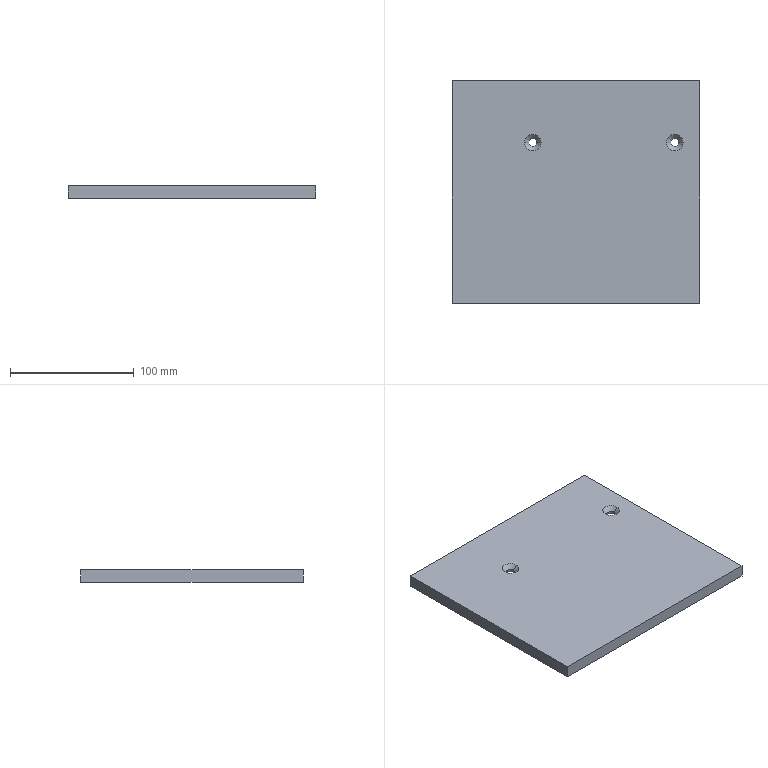Part | STEP file | 001-004-Feeding mechanism shaft slideway base plate | 1 solid | 20 faces | box 200 x 180 x 10 mm | volume 352263 mm3 | cylinder 8 | plane 8 | cone 4 | commonest cylinder face diameters 6.6 x4 30 x4
STEP:
#1=CARTESIAN_POINT('',(0.,0.,0.));
#2=DIRECTION('',(0.,0.,1.));
#3=DIRECTION('',(1.,0.,0.));
#4=AXIS2_PLACEMENT_3D('',#1,#2,#3);
#5=CARTESIAN_POINT('',(-31.7,40.,6.58));
#6=VERTEX_POINT('',#5);
#7=CARTESIAN_POINT('',(-28.28,40.,10.));
#8=VERTEX_POINT('',#7);
#9=CARTESIAN_POINT('',(-28.28,40.,10.));
#10=DIRECTION('',(0.7071,0.,0.7071));
#11=VECTOR('',#10,1.);
#12=LINE('',#9,#11);
#13=CARTESIAN_POINT('',(-35.,40.,10.));
#14=DIRECTION('',(0.,0.,1.));
#15=DIRECTION('',(1.,0.,0.));
#16=AXIS2_PLACEMENT_3D('',#13,#14,#15);
#17=CONICAL_SURFACE('',#16,6.72,0.7854);
#18=CARTESIAN_POINT('',(6.283,0.));
#19=DIRECTION('',(0.,1.));
#20=VECTOR('',#19,1.);
#21=LINE('',#18,#20);
#22=(GEOMETRIC_REPRESENTATION_CONTEXT(2)PARAMETRIC_REPRESENTATION_CONTEXT()REPRESENTATION_CONTEXT('',''));
#23=DEFINITIONAL_REPRESENTATION('',(#21),#22);
#24=PCURVE('',#17,#23);
#25=CARTESIAN_POINT('',(-35.,40.,10.));
#26=DIRECTION('',(0.,0.,1.));
#27=DIRECTION('',(1.,0.,0.));
#28=AXIS2_PLACEMENT_3D('',#25,#26,#27);
#29=CONICAL_SURFACE('',#28,6.72,0.7854);
#30=CARTESIAN_POINT('',(0.,0.));
#31=DIRECTION('',(0.,1.));
#32=VECTOR('',#31,1.);
#33=LINE('',#30,#32);
#34=(GEOMETRIC_REPRESENTATION_CONTEXT(2)PARAMETRIC_REPRESENTATION_CONTEXT()REPRESENTATION_CONTEXT('',''));
#35=DEFINITIONAL_REPRESENTATION('',(#33),#34);
#36=PCURVE('',#29,#35);
#37=SURFACE_CURVE('',#12,(#24,#36),.PCURVE_S1.);
#38=EDGE_CURVE('',#6,#8,#37,.T.);
#39=ORIENTED_EDGE('',*,*,#38,.T.);
#40=CARTESIAN_POINT('',(-41.72,40.,10.));
#41=VERTEX_POINT('',#40);
#42=CARTESIAN_POINT('',(-35.,40.,10.));
#43=DIRECTION('',(0.,0.,1.));
#44=DIRECTION('',(1.,0.,0.));
#45=AXIS2_PLACEMENT_3D('',#42,#43,#44);
#46=CIRCLE('',#45,6.72);
#47=CARTESIAN_POINT('',(0.,0.));
#48=DIRECTION('',(1.,0.));
#49=VECTOR('',#48,1.);
#50=LINE('',#47,#49);
#51=(GEOMETRIC_REPRESENTATION_CONTEXT(2)PARAMETRIC_REPRESENTATION_CONTEXT()REPRESENTATION_CONTEXT('',''));
#52=DEFINITIONAL_REPRESENTATION('',(#50),#51);
#53=PCURVE('',#17,#52);
#54=CARTESIAN_POINT('',(0.,0.,10.));
#55=DIRECTION('',(0.,0.,1.));
#56=DIRECTION('',(1.,0.,0.));
#57=AXIS2_PLACEMENT_3D('',#54,#55,#56);
#58=PLANE('',#57);
#59=CARTESIAN_POINT('',(-35.,40.));
#60=DIRECTION('',(1.,0.));
#61=AXIS2_PLACEMENT_2D('',#59,#60);
#62=CIRCLE('',#61,6.72);
#63=(GEOMETRIC_REPRESENTATION_CONTEXT(2)PARAMETRIC_REPRESENTATION_CONTEXT()REPRESENTATION_CONTEXT('',''));
#64=DEFINITIONAL_REPRESENTATION('',(#62),#63);
#65=PCURVE('',#58,#64);
#66=SURFACE_CURVE('',#46,(#53,#65),.PCURVE_S1.);
#67=EDGE_CURVE('',#41,#8,#66,.T.);
#68=ORIENTED_EDGE('',*,*,#67,.F.);
#69=CARTESIAN_POINT('',(-38.3,40.,6.58));
#70=VERTEX_POINT('',#69);
#71=CARTESIAN_POINT('',(-41.72,40.,10.));
#72=DIRECTION('',(-0.7071,0.,0.7071));
#73=VECTOR('',#72,1.);
#74=LINE('',#71,#73);
#75=CARTESIAN_POINT('',(3.142,0.));
#76=DIRECTION('',(0.,1.));
#77=VECTOR('',#76,1.);
#78=LINE('',#75,#77);
#79=(GEOMETRIC_REPRESENTATION_CONTEXT(2)PARAMETRIC_REPRESENTATION_CONTEXT()REPRESENTATION_CONTEXT('',''));
#80=DEFINITIONAL_REPRESENTATION('',(#78),#79);
#81=PCURVE('',#17,#80);
#82=CARTESIAN_POINT('',(3.142,0.));
#83=DIRECTION('',(0.,1.));
#84=VECTOR('',#83,1.);
#85=LINE('',#82,#84);
#86=(GEOMETRIC_REPRESENTATION_CONTEXT(2)PARAMETRIC_REPRESENTATION_CONTEXT()REPRESENTATION_CONTEXT('',''));
#87=DEFINITIONAL_REPRESENTATION('',(#85),#86);
#88=PCURVE('',#29,#87);
#89=SURFACE_CURVE('',#74,(#81,#88),.PCURVE_S1.);
#90=EDGE_CURVE('',#70,#41,#89,.T.);
#91=ORIENTED_EDGE('',*,*,#90,.F.);
#92=CARTESIAN_POINT('',(-35.,40.,6.58));
#93=DIRECTION('',(0.,0.,1.));
#94=DIRECTION('',(1.,0.,0.));
#95=AXIS2_PLACEMENT_3D('',#92,#93,#94);
#96=CIRCLE('',#95,3.3);
#97=CARTESIAN_POINT('',(0.,-3.42));
#98=DIRECTION('',(1.,0.));
#99=VECTOR('',#98,1.);
#100=LINE('',#97,#99);
#101=(GEOMETRIC_REPRESENTATION_CONTEXT(2)PARAMETRIC_REPRESENTATION_CONTEXT()REPRESENTATION_CONTEXT('',''));
#102=DEFINITIONAL_REPRESENTATION('',(#100),#101);
#103=PCURVE('',#17,#102);
#104=CARTESIAN_POINT('',(-35.,40.,10.));
#105=DIRECTION('',(0.,0.,1.));
#106=DIRECTION('',(1.,0.,0.));
#107=AXIS2_PLACEMENT_3D('',#104,#105,#106);
#108=CYLINDRICAL_SURFACE('',#107,3.3);
#109=CARTESIAN_POINT('',(0.,-3.42));
#110=DIRECTION('',(1.,0.));
#111=VECTOR('',#110,1.);
#112=LINE('',#109,#111);
#113=(GEOMETRIC_REPRESENTATION_CONTEXT(2)PARAMETRIC_REPRESENTATION_CONTEXT()REPRESENTATION_CONTEXT('',''));
#114=DEFINITIONAL_REPRESENTATION('',(#112),#113);
#115=PCURVE('',#108,#114);
#116=SURFACE_CURVE('',#96,(#103,#115),.PCURVE_S1.);
#117=EDGE_CURVE('',#70,#6,#116,.T.);
#118=ORIENTED_EDGE('',*,*,#117,.T.);
#119=EDGE_LOOP('',(#39,#68,#91,#118));
#120=FACE_BOUND('',#119,.F.);
#121=ADVANCED_FACE('',(#120),#17,.F.);
#122=CARTESIAN_POINT('',(-31.7,40.,5.));
#123=VERTEX_POINT('',#122);
#124=CARTESIAN_POINT('',(-31.7,40.,10.));
#125=DIRECTION('',(0.,0.,1.));
#126=VECTOR('',#125,1.);
#127=LINE('',#124,#126);
#128=CARTESIAN_POINT('',(6.283,0.));
#129=DIRECTION('',(0.,1.));
#130=VECTOR('',#129,1.);
#131=LINE('',#128,#130);
#132=(GEOMETRIC_REPRESENTATION_CONTEXT(2)PARAMETRIC_REPRESENTATION_CONTEXT()REPRESENTATION_CONTEXT('',''));
#133=DEFINITIONAL_REPRESENTATION('',(#131),#132);
#134=PCURVE('',#108,#133);
#135=CARTESIAN_POINT('',(-35.,40.,10.));
#136=DIRECTION('',(0.,0.,1.));
#137=DIRECTION('',(1.,0.,0.));
#138=AXIS2_PLACEMENT_3D('',#135,#136,#137);
#139=CYLINDRICAL_SURFACE('',#138,3.3);
#140=CARTESIAN_POINT('',(0.,0.));
#141=DIRECTION('',(0.,1.));
#142=VECTOR('',#141,1.);
#143=LINE('',#140,#142);
#144=(GEOMETRIC_REPRESENTATION_CONTEXT(2)PARAMETRIC_REPRESENTATION_CONTEXT()REPRESENTATION_CONTEXT('',''));
#145=DEFINITIONAL_REPRESENTATION('',(#143),#144);
#146=PCURVE('',#139,#145);
#147=SURFACE_CURVE('',#127,(#134,#146),.PCURVE_S1.);
#148=EDGE_CURVE('',#123,#6,#147,.T.);
#149=ORIENTED_EDGE('',*,*,#148,.T.);
#150=ORIENTED_EDGE('',*,*,#117,.F.);
#151=CARTESIAN_POINT('',(-38.3,40.,5.));
#152=VERTEX_POINT('',#151);
#153=CARTESIAN_POINT('',(-38.3,40.,10.));
#154=DIRECTION('',(0.,0.,1.));
#155=VECTOR('',#154,1.);
#156=LINE('',#153,#155);
#157=CARTESIAN_POINT('',(3.142,0.));
#158=DIRECTION('',(0.,1.));
#159=VECTOR('',#158,1.);
#160=LINE('',#157,#159);
#161=(GEOMETRIC_REPRESENTATION_CONTEXT(2)PARAMETRIC_REPRESENTATION_CONTEXT()REPRESENTATION_CONTEXT('',''));
#162=DEFINITIONAL_REPRESENTATION('',(#160),#161);
#163=PCURVE('',#108,#162);
#164=CARTESIAN_POINT('',(3.142,0.));
#165=DIRECTION('',(0.,1.));
#166=VECTOR('',#165,1.);
#167=LINE('',#164,#166);
#168=(GEOMETRIC_REPRESENTATION_CONTEXT(2)PARAMETRIC_REPRESENTATION_CONTEXT()REPRESENTATION_CONTEXT('',''));
#169=DEFINITIONAL_REPRESENTATION('',(#167),#168);
#170=PCURVE('',#139,#169);
#171=SURFACE_CURVE('',#156,(#163,#170),.PCURVE_S1.);
#172=EDGE_CURVE('',#152,#70,#171,.T.);
#173=ORIENTED_EDGE('',*,*,#172,.F.);
#174=CARTESIAN_POINT('',(-35.,40.,5.));
#175=DIRECTION('',(0.,0.,-1.));
#176=DIRECTION('',(-1.,0.,0.));
#177=AXIS2_PLACEMENT_3D('',#174,#175,#176);
#178=CIRCLE('',#177,3.3);
#179=CARTESIAN_POINT('',(9.425,-5.));
#180=DIRECTION('',(-1.,0.));
#181=VECTOR('',#180,1.);
#182=LINE('',#179,#181);
#183=(GEOMETRIC_REPRESENTATION_CONTEXT(2)PARAMETRIC_REPRESENTATION_CONTEXT()REPRESENTATION_CONTEXT('',''));
#184=DEFINITIONAL_REPRESENTATION('',(#182),#183);
#185=PCURVE('',#108,#184);
#186=CARTESIAN_POINT('',(-35.,40.,5.));
#187=DIRECTION('',(0.,0.,-1.));
#188=DIRECTION('',(-1.,0.,0.));
#189=AXIS2_PLACEMENT_3D('',#186,#187,#188);
#190=PLANE('',#189);
#191=CARTESIAN_POINT('',(0.,0.));
#192=DIRECTION('',(1.,0.));
#193=AXIS2_PLACEMENT_2D('',#191,#192);
#194=CIRCLE('',#193,3.3);
#195=(GEOMETRIC_REPRESENTATION_CONTEXT(2)PARAMETRIC_REPRESENTATION_CONTEXT()REPRESENTATION_CONTEXT('',''));
#196=DEFINITIONAL_REPRESENTATION('',(#194),#195);
#197=PCURVE('',#190,#196);
#198=SURFACE_CURVE('',#178,(#185,#197),.PCURVE_S1.);
#199=EDGE_CURVE('',#123,#152,#198,.T.);
#200=ORIENTED_EDGE('',*,*,#199,.F.);
#201=EDGE_LOOP('',(#149,#150,#173,#200));
#202=FACE_BOUND('',#201,.F.);
#203=ADVANCED_FACE('',(#202),#108,.F.);
#204=CARTESIAN_POINT('',(83.3,40.,6.58));
#205=VERTEX_POINT('',#204);
#206=CARTESIAN_POINT('',(86.72,40.,10.));
#207=VERTEX_POINT('',#206);
#208=CARTESIAN_POINT('',(86.72,40.,10.));
#209=DIRECTION('',(0.7071,0.,0.7071));
#210=VECTOR('',#209,1.);
#211=LINE('',#208,#210);
#212=CARTESIAN_POINT('',(80.,40.,10.));
#213=DIRECTION('',(0.,0.,1.));
#214=DIRECTION('',(1.,0.,0.));
#215=AXIS2_PLACEMENT_3D('',#212,#213,#214);
#216=CONICAL_SURFACE('',#215,6.72,0.7854);
#217=CARTESIAN_POINT('',(6.283,0.));
#218=DIRECTION('',(0.,1.));
#219=VECTOR('',#218,1.);
#220=LINE('',#217,#219);
#221=(GEOMETRIC_REPRESENTATION_CONTEXT(2)PARAMETRIC_REPRESENTATION_CONTEXT()REPRESENTATION_CONTEXT('',''));
#222=DEFINITIONAL_REPRESENTATION('',(#220),#221);
#223=PCURVE('',#216,#222);
#224=CARTESIAN_POINT('',(80.,40.,10.));
#225=DIRECTION('',(0.,0.,1.));
#226=DIRECTION('',(1.,0.,0.));
#227=AXIS2_PLACEMENT_3D('',#224,#225,#226);
#228=CONICAL_SURFACE('',#227,6.72,0.7854);
#229=CARTESIAN_POINT('',(0.,0.));
#230=DIRECTION('',(0.,1.));
#231=VECTOR('',#230,1.);
#232=LINE('',#229,#231);
#233=(GEOMETRIC_REPRESENTATION_CONTEXT(2)PARAMETRIC_REPRESENTATION_CONTEXT()REPRESENTATION_CONTEXT('',''));
#234=DEFINITIONAL_REPRESENTATION('',(#232),#233);
#235=PCURVE('',#228,#234);
#236=SURFACE_CURVE('',#211,(#223,#235),.PCURVE_S1.);
#237=EDGE_CURVE('',#205,#207,#236,.T.);
#238=ORIENTED_EDGE('',*,*,#237,.T.);
#239=CARTESIAN_POINT('',(73.28,40.,10.));
#240=VERTEX_POINT('',#239);
#241=CARTESIAN_POINT('',(80.,40.,10.));
#242=DIRECTION('',(0.,0.,1.));
#243=DIRECTION('',(1.,0.,0.));
#244=AXIS2_PLACEMENT_3D('',#241,#242,#243);
#245=CIRCLE('',#244,6.72);
#246=CARTESIAN_POINT('',(0.,0.));
#247=DIRECTION('',(1.,0.));
#248=VECTOR('',#247,1.);
#249=LINE('',#246,#248);
#250=(GEOMETRIC_REPRESENTATION_CONTEXT(2)PARAMETRIC_REPRESENTATION_CONTEXT()REPRESENTATION_CONTEXT('',''));
#251=DEFINITIONAL_REPRESENTATION('',(#249),#250);
#252=PCURVE('',#216,#251);
#253=CARTESIAN_POINT('',(80.,40.));
#254=DIRECTION('',(1.,0.));
#255=AXIS2_PLACEMENT_2D('',#253,#254);
#256=CIRCLE('',#255,6.72);
#257=(GEOMETRIC_REPRESENTATION_CONTEXT(2)PARAMETRIC_REPRESENTATION_CONTEXT()REPRESENTATION_CONTEXT('',''));
#258=DEFINITIONAL_REPRESENTATION('',(#256),#257);
#259=PCURVE('',#58,#258);
#260=SURFACE_CURVE('',#245,(#252,#259),.PCURVE_S1.);
#261=EDGE_CURVE('',#240,#207,#260,.T.);
#262=ORIENTED_EDGE('',*,*,#261,.F.);
#263=CARTESIAN_POINT('',(76.7,40.,6.58));
#264=VERTEX_POINT('',#263);
#265=CARTESIAN_POINT('',(73.28,40.,10.));
#266=DIRECTION('',(-0.7071,0.,0.7071));
#267=VECTOR('',#266,1.);
#268=LINE('',#265,#267);
#269=CARTESIAN_POINT('',(3.142,0.));
#270=DIRECTION('',(0.,1.));
#271=VECTOR('',#270,1.);
#272=LINE('',#269,#271);
#273=(GEOMETRIC_REPRESENTATION_CONTEXT(2)PARAMETRIC_REPRESENTATION_CONTEXT()REPRESENTATION_CONTEXT('',''));
#274=DEFINITIONAL_REPRESENTATION('',(#272),#273);
#275=PCURVE('',#216,#274);
#276=CARTESIAN_POINT('',(3.142,0.));
#277=DIRECTION('',(0.,1.));
#278=VECTOR('',#277,1.);
#279=LINE('',#276,#278);
#280=(GEOMETRIC_REPRESENTATION_CONTEXT(2)PARAMETRIC_REPRESENTATION_CONTEXT()REPRESENTATION_CONTEXT('',''));
#281=DEFINITIONAL_REPRESENTATION('',(#279),#280);
#282=PCURVE('',#228,#281);
#283=SURFACE_CURVE('',#268,(#275,#282),.PCURVE_S1.);
#284=EDGE_CURVE('',#264,#240,#283,.T.);
#285=ORIENTED_EDGE('',*,*,#284,.F.);
#286=CARTESIAN_POINT('',(80.,40.,6.58));
#287=DIRECTION('',(0.,0.,1.));
#288=DIRECTION('',(1.,0.,0.));
#289=AXIS2_PLACEMENT_3D('',#286,#287,#288);
#290=CIRCLE('',#289,3.3);
#291=CARTESIAN_POINT('',(0.,-3.42));
#292=DIRECTION('',(1.,0.));
#293=VECTOR('',#292,1.);
#294=LINE('',#291,#293);
#295=(GEOMETRIC_REPRESENTATION_CONTEXT(2)PARAMETRIC_REPRESENTATION_CONTEXT()REPRESENTATION_CONTEXT('',''));
#296=DEFINITIONAL_REPRESENTATION('',(#294),#295);
#297=PCURVE('',#216,#296);
#298=CARTESIAN_POINT('',(80.,40.,10.));
#299=DIRECTION('',(0.,0.,1.));
#300=DIRECTION('',(1.,0.,0.));
#301=AXIS2_PLACEMENT_3D('',#298,#299,#300);
#302=CYLINDRICAL_SURFACE('',#301,3.3);
#303=CARTESIAN_POINT('',(0.,-3.42));
#304=DIRECTION('',(1.,0.));
#305=VECTOR('',#304,1.);
#306=LINE('',#303,#305);
#307=(GEOMETRIC_REPRESENTATION_CONTEXT(2)PARAMETRIC_REPRESENTATION_CONTEXT()REPRESENTATION_CONTEXT('',''));
#308=DEFINITIONAL_REPRESENTATION('',(#306),#307);
#309=PCURVE('',#302,#308);
#310=SURFACE_CURVE('',#290,(#297,#309),.PCURVE_S1.);
#311=EDGE_CURVE('',#264,#205,#310,.T.);
#312=ORIENTED_EDGE('',*,*,#311,.T.);
#313=EDGE_LOOP('',(#238,#262,#285,#312));
#314=FACE_BOUND('',#313,.F.);
#315=ADVANCED_FACE('',(#314),#216,.F.);
#316=CARTESIAN_POINT('',(83.3,40.,5.));
#317=VERTEX_POINT('',#316);
#318=CARTESIAN_POINT('',(83.3,40.,10.));
#319=DIRECTION('',(0.,0.,1.));
#320=VECTOR('',#319,1.);
#321=LINE('',#318,#320);
#322=CARTESIAN_POINT('',(6.283,0.));
#323=DIRECTION('',(0.,1.));
#324=VECTOR('',#323,1.);
#325=LINE('',#322,#324);
#326=(GEOMETRIC_REPRESENTATION_CONTEXT(2)PARAMETRIC_REPRESENTATION_CONTEXT()REPRESENTATION_CONTEXT('',''));
#327=DEFINITIONAL_REPRESENTATION('',(#325),#326);
#328=PCURVE('',#302,#327);
#329=CARTESIAN_POINT('',(80.,40.,10.));
#330=DIRECTION('',(0.,0.,1.));
#331=DIRECTION('',(1.,0.,0.));
#332=AXIS2_PLACEMENT_3D('',#329,#330,#331);
#333=CYLINDRICAL_SURFACE('',#332,3.3);
#334=CARTESIAN_POINT('',(0.,0.));
#335=DIRECTION('',(0.,1.));
#336=VECTOR('',#335,1.);
#337=LINE('',#334,#336);
#338=(GEOMETRIC_REPRESENTATION_CONTEXT(2)PARAMETRIC_REPRESENTATION_CONTEXT()REPRESENTATION_CONTEXT('',''));
#339=DEFINITIONAL_REPRESENTATION('',(#337),#338);
#340=PCURVE('',#333,#339);
#341=SURFACE_CURVE('',#321,(#328,#340),.PCURVE_S1.);
#342=EDGE_CURVE('',#317,#205,#341,.T.);
#343=ORIENTED_EDGE('',*,*,#342,.T.);
#344=ORIENTED_EDGE('',*,*,#311,.F.);
#345=CARTESIAN_POINT('',(76.7,40.,5.));
#346=VERTEX_POINT('',#345);
#347=CARTESIAN_POINT('',(76.7,40.,10.));
#348=DIRECTION('',(0.,0.,1.));
#349=VECTOR('',#348,1.);
#350=LINE('',#347,#349);
#351=CARTESIAN_POINT('',(3.142,0.));
#352=DIRECTION('',(0.,1.));
#353=VECTOR('',#352,1.);
#354=LINE('',#351,#353);
#355=(GEOMETRIC_REPRESENTATION_CONTEXT(2)PARAMETRIC_REPRESENTATION_CONTEXT()REPRESENTATION_CONTEXT('',''));
#356=DEFINITIONAL_REPRESENTATION('',(#354),#355);
#357=PCURVE('',#302,#356);
#358=CARTESIAN_POINT('',(3.142,0.));
#359=DIRECTION('',(0.,1.));
#360=VECTOR('',#359,1.);
#361=LINE('',#358,#360);
#362=(GEOMETRIC_REPRESENTATION_CONTEXT(2)PARAMETRIC_REPRESENTATION_CONTEXT()REPRESENTATION_CONTEXT('',''));
#363=DEFINITIONAL_REPRESENTATION('',(#361),#362);
#364=PCURVE('',#333,#363);
#365=SURFACE_CURVE('',#350,(#357,#364),.PCURVE_S1.);
#366=EDGE_CURVE('',#346,#264,#365,.T.);
#367=ORIENTED_EDGE('',*,*,#366,.F.);
#368=CARTESIAN_POINT('',(80.,40.,5.));
#369=DIRECTION('',(0.,0.,-1.));
#370=DIRECTION('',(-1.,0.,0.));
#371=AXIS2_PLACEMENT_3D('',#368,#369,#370);
#372=CIRCLE('',#371,3.3);
#373=CARTESIAN_POINT('',(9.425,-5.));
#374=DIRECTION('',(-1.,0.));
#375=VECTOR('',#374,1.);
#376=LINE('',#373,#375);
#377=(GEOMETRIC_REPRESENTATION_CONTEXT(2)PARAMETRIC_REPRESENTATION_CONTEXT()REPRESENTATION_CONTEXT('',''));
#378=DEFINITIONAL_REPRESENTATION('',(#376),#377);
#379=PCURVE('',#302,#378);
#380=CARTESIAN_POINT('',(80.,40.,5.));
#381=DIRECTION('',(0.,0.,-1.));
#382=DIRECTION('',(-1.,0.,0.));
#383=AXIS2_PLACEMENT_3D('',#380,#381,#382);
#384=PLANE('',#383);
#385=CARTESIAN_POINT('',(0.,0.));
#386=DIRECTION('',(1.,0.));
#387=AXIS2_PLACEMENT_2D('',#385,#386);
#388=CIRCLE('',#387,3.3);
#389=(GEOMETRIC_REPRESENTATION_CONTEXT(2)PARAMETRIC_REPRESENTATION_CONTEXT()REPRESENTATION_CONTEXT('',''));
#390=DEFINITIONAL_REPRESENTATION('',(#388),#389);
#391=PCURVE('',#384,#390);
#392=SURFACE_CURVE('',#372,(#379,#391),.PCURVE_S1.);
#393=EDGE_CURVE('',#317,#346,#392,.T.);
#394=ORIENTED_EDGE('',*,*,#393,.F.);
#395=EDGE_LOOP('',(#343,#344,#367,#394));
#396=FACE_BOUND('',#395,.F.);
#397=ADVANCED_FACE('',(#396),#302,.F.);
#398=CARTESIAN_POINT('',(-50.,40.,5.));
#399=VERTEX_POINT('',#398);
#400=CARTESIAN_POINT('',(-50.,40.,0.));
#401=VERTEX_POINT('',#400);
#402=CARTESIAN_POINT('',(-50.,40.,5.));
#403=DIRECTION('',(0.,0.,-1.));
#404=VECTOR('',#403,1.);
#405=LINE('',#402,#404);
#406=CARTESIAN_POINT('',(-35.,40.,5.));
#407=DIRECTION('',(0.,0.,-1.));
#408=DIRECTION('',(-1.,0.,0.));
#409=AXIS2_PLACEMENT_3D('',#406,#407,#408);
#410=CYLINDRICAL_SURFACE('',#409,15.);
#411=CARTESIAN_POINT('',(6.283,0.));
#412=DIRECTION('',(0.,1.));
#413=VECTOR('',#412,1.);
#414=LINE('',#411,#413);
#415=(GEOMETRIC_REPRESENTATION_CONTEXT(2)PARAMETRIC_REPRESENTATION_CONTEXT()REPRESENTATION_CONTEXT('',''));
#416=DEFINITIONAL_REPRESENTATION('',(#414),#415);
#417=PCURVE('',#410,#416);
#418=CARTESIAN_POINT('',(-35.,40.,5.));
#419=DIRECTION('',(0.,0.,-1.));
#420=DIRECTION('',(-1.,0.,0.));
#421=AXIS2_PLACEMENT_3D('',#418,#419,#420);
#422=CYLINDRICAL_SURFACE('',#421,15.);
#423=CARTESIAN_POINT('',(0.,0.));
#424=DIRECTION('',(0.,1.));
#425=VECTOR('',#424,1.);
#426=LINE('',#423,#425);
#427=(GEOMETRIC_REPRESENTATION_CONTEXT(2)PARAMETRIC_REPRESENTATION_CONTEXT()REPRESENTATION_CONTEXT('',''));
#428=DEFINITIONAL_REPRESENTATION('',(#426),#427);
#429=PCURVE('',#422,#428);
#430=SURFACE_CURVE('',#405,(#417,#429),.PCURVE_S1.);
#431=EDGE_CURVE('',#399,#401,#430,.T.);
#432=ORIENTED_EDGE('',*,*,#431,.T.);
#433=CARTESIAN_POINT('',(-20.,40.,0.));
#434=VERTEX_POINT('',#433);
#435=CARTESIAN_POINT('',(-35.,40.,0.));
#436=DIRECTION('',(0.,0.,-1.));
#437=DIRECTION('',(-1.,0.,0.));
#438=AXIS2_PLACEMENT_3D('',#435,#436,#437);
#439=CIRCLE('',#438,15.);
#440=CARTESIAN_POINT('',(0.,5.));
#441=DIRECTION('',(1.,0.));
#442=VECTOR('',#441,1.);
#443=LINE('',#440,#442);
#444=(GEOMETRIC_REPRESENTATION_CONTEXT(2)PARAMETRIC_REPRESENTATION_CONTEXT()REPRESENTATION_CONTEXT('',''));
#445=DEFINITIONAL_REPRESENTATION('',(#443),#444);
#446=PCURVE('',#410,#445);
#447=CARTESIAN_POINT('',(0.,0.,0.));
#448=DIRECTION('',(0.,0.,1.));
#449=DIRECTION('',(1.,0.,0.));
#450=AXIS2_PLACEMENT_3D('',#447,#448,#449);
#451=PLANE('',#450);
#452=CARTESIAN_POINT('',(-50.,40.));
#453=CARTESIAN_POINT('',(-50.,65.981));
#454=CARTESIAN_POINT('',(-27.5,52.99));
#455=CARTESIAN_POINT('',(-5.,40.));
#456=CARTESIAN_POINT('',(-27.5,27.01));
#457=CARTESIAN_POINT('',(-50.,14.019));
#458=CARTESIAN_POINT('',(-50.,40.));
#459=(BOUNDED_CURVE()B_SPLINE_CURVE(2,(#452,#453,#454,#455,#456,#457,#458),.UNSPECIFIED.,.T.,.F.)B_SPLINE_CURVE_WITH_KNOTS((1,2,2,2,2,1),(-2.094,0.,2.094,4.189,6.283,8.378),.UNSPECIFIED.)CURVE()GEOMETRIC_REPRESENTATION_ITEM()RATIONAL_B_SPLINE_CURVE((1.,0.5,1.,0.5,1.,0.5,1.))REPRESENTATION_ITEM(''));
#460=(GEOMETRIC_REPRESENTATION_CONTEXT(2)PARAMETRIC_REPRESENTATION_CONTEXT()REPRESENTATION_CONTEXT('',''));
#461=DEFINITIONAL_REPRESENTATION('',(#459),#460);
#462=PCURVE('',#451,#461);
#463=SURFACE_CURVE('',#439,(#446,#462),.PCURVE_S1.);
#464=EDGE_CURVE('',#434,#401,#463,.T.);
#465=ORIENTED_EDGE('',*,*,#464,.F.);
#466=CARTESIAN_POINT('',(-20.,40.,5.));
#467=VERTEX_POINT('',#466);
#468=CARTESIAN_POINT('',(-20.,40.,5.));
#469=DIRECTION('',(0.,0.,-1.));
#470=VECTOR('',#469,1.);
#471=LINE('',#468,#470);
#472=CARTESIAN_POINT('',(3.142,0.));
#473=DIRECTION('',(0.,1.));
#474=VECTOR('',#473,1.);
#475=LINE('',#472,#474);
#476=(GEOMETRIC_REPRESENTATION_CONTEXT(2)PARAMETRIC_REPRESENTATION_CONTEXT()REPRESENTATION_CONTEXT('',''));
#477=DEFINITIONAL_REPRESENTATION('',(#475),#476);
#478=PCURVE('',#410,#477);
#479=CARTESIAN_POINT('',(3.142,0.));
#480=DIRECTION('',(0.,1.));
#481=VECTOR('',#480,1.);
#482=LINE('',#479,#481);
#483=(GEOMETRIC_REPRESENTATION_CONTEXT(2)PARAMETRIC_REPRESENTATION_CONTEXT()REPRESENTATION_CONTEXT('',''));
#484=DEFINITIONAL_REPRESENTATION('',(#482),#483);
#485=PCURVE('',#422,#484);
#486=SURFACE_CURVE('',#471,(#478,#485),.PCURVE_S1.);
#487=EDGE_CURVE('',#467,#434,#486,.T.);
#488=ORIENTED_EDGE('',*,*,#487,.F.);
#489=CARTESIAN_POINT('',(-35.,40.,5.));
#490=DIRECTION('',(0.,0.,-1.));
#491=DIRECTION('',(-1.,0.,0.));
#492=AXIS2_PLACEMENT_3D('',#489,#490,#491);
#493=CIRCLE('',#492,15.);
#494=CARTESIAN_POINT('',(0.,0.));
#495=DIRECTION('',(1.,0.));
#496=VECTOR('',#495,1.);
#497=LINE('',#494,#496);
#498=(GEOMETRIC_REPRESENTATION_CONTEXT(2)PARAMETRIC_REPRESENTATION_CONTEXT()REPRESENTATION_CONTEXT('',''));
#499=DEFINITIONAL_REPRESENTATION('',(#497),#498);
#500=PCURVE('',#410,#499);
#501=CARTESIAN_POINT('',(0.,0.));
#502=DIRECTION('',(1.,0.));
#503=AXIS2_PLACEMENT_2D('',#501,#502);
#504=CIRCLE('',#503,15.);
#505=(GEOMETRIC_REPRESENTATION_CONTEXT(2)PARAMETRIC_REPRESENTATION_CONTEXT()REPRESENTATION_CONTEXT('',''));
#506=DEFINITIONAL_REPRESENTATION('',(#504),#505);
#507=PCURVE('',#190,#506);
#508=SURFACE_CURVE('',#493,(#500,#507),.PCURVE_S1.);
#509=EDGE_CURVE('',#467,#399,#508,.T.);
#510=ORIENTED_EDGE('',*,*,#509,.T.);
#511=EDGE_LOOP('',(#432,#465,#488,#510));
#512=FACE_BOUND('',#511,.F.);
#513=ADVANCED_FACE('',(#512),#410,.F.);
#514=CARTESIAN_POINT('',(65.,40.,5.));
#515=VERTEX_POINT('',#514);
#516=CARTESIAN_POINT('',(65.,40.,0.));
#517=VERTEX_POINT('',#516);
#518=CARTESIAN_POINT('',(65.,40.,5.));
#519=DIRECTION('',(0.,0.,-1.));
#520=VECTOR('',#519,1.);
#521=LINE('',#518,#520);
#522=CARTESIAN_POINT('',(80.,40.,5.));
#523=DIRECTION('',(0.,0.,-1.));
#524=DIRECTION('',(-1.,0.,0.));
#525=AXIS2_PLACEMENT_3D('',#522,#523,#524);
#526=CYLINDRICAL_SURFACE('',#525,15.);
#527=CARTESIAN_POINT('',(6.283,0.));
#528=DIRECTION('',(0.,1.));
#529=VECTOR('',#528,1.);
#530=LINE('',#527,#529);
#531=(GEOMETRIC_REPRESENTATION_CONTEXT(2)PARAMETRIC_REPRESENTATION_CONTEXT()REPRESENTATION_CONTEXT('',''));
#532=DEFINITIONAL_REPRESENTATION('',(#530),#531);
#533=PCURVE('',#526,#532);
#534=CARTESIAN_POINT('',(80.,40.,5.));
#535=DIRECTION('',(0.,0.,-1.));
#536=DIRECTION('',(-1.,0.,0.));
#537=AXIS2_PLACEMENT_3D('',#534,#535,#536);
#538=CYLINDRICAL_SURFACE('',#537,15.);
#539=CARTESIAN_POINT('',(0.,0.));
#540=DIRECTION('',(0.,1.));
#541=VECTOR('',#540,1.);
#542=LINE('',#539,#541);
#543=(GEOMETRIC_REPRESENTATION_CONTEXT(2)PARAMETRIC_REPRESENTATION_CONTEXT()REPRESENTATION_CONTEXT('',''));
#544=DEFINITIONAL_REPRESENTATION('',(#542),#543);
#545=PCURVE('',#538,#544);
#546=SURFACE_CURVE('',#521,(#533,#545),.PCURVE_S1.);
#547=EDGE_CURVE('',#515,#517,#546,.T.);
#548=ORIENTED_EDGE('',*,*,#547,.T.);
#549=CARTESIAN_POINT('',(95.,40.,0.));
#550=VERTEX_POINT('',#549);
#551=CARTESIAN_POINT('',(80.,40.,0.));
#552=DIRECTION('',(0.,0.,-1.));
#553=DIRECTION('',(-1.,0.,0.));
#554=AXIS2_PLACEMENT_3D('',#551,#552,#553);
#555=CIRCLE('',#554,15.);
#556=CARTESIAN_POINT('',(0.,5.));
#557=DIRECTION('',(1.,0.));
#558=VECTOR('',#557,1.);
#559=LINE('',#556,#558);
#560=(GEOMETRIC_REPRESENTATION_CONTEXT(2)PARAMETRIC_REPRESENTATION_CONTEXT()REPRESENTATION_CONTEXT('',''));
#561=DEFINITIONAL_REPRESENTATION('',(#559),#560);
#562=PCURVE('',#526,#561);
#563=CARTESIAN_POINT('',(65.,40.));
#564=CARTESIAN_POINT('',(65.,65.981));
#565=CARTESIAN_POINT('',(87.5,52.99));
#566=CARTESIAN_POINT('',(110.,40.));
#567=CARTESIAN_POINT('',(87.5,27.01));
#568=CARTESIAN_POINT('',(65.,14.019));
#569=CARTESIAN_POINT('',(65.,40.));
#570=(BOUNDED_CURVE()B_SPLINE_CURVE(2,(#563,#564,#565,#566,#567,#568,#569),.UNSPECIFIED.,.T.,.F.)B_SPLINE_CURVE_WITH_KNOTS((1,2,2,2,2,1),(-2.094,0.,2.094,4.189,6.283,8.378),.UNSPECIFIED.)CURVE()GEOMETRIC_REPRESENTATION_ITEM()RATIONAL_B_SPLINE_CURVE((1.,0.5,1.,0.5,1.,0.5,1.))REPRESENTATION_ITEM(''));
#571=(GEOMETRIC_REPRESENTATION_CONTEXT(2)PARAMETRIC_REPRESENTATION_CONTEXT()REPRESENTATION_CONTEXT('',''));
#572=DEFINITIONAL_REPRESENTATION('',(#570),#571);
#573=PCURVE('',#451,#572);
#574=SURFACE_CURVE('',#555,(#562,#573),.PCURVE_S1.);
#575=EDGE_CURVE('',#550,#517,#574,.T.);
#576=ORIENTED_EDGE('',*,*,#575,.F.);
#577=CARTESIAN_POINT('',(95.,40.,5.));
#578=VERTEX_POINT('',#577);
#579=CARTESIAN_POINT('',(95.,40.,5.));
#580=DIRECTION('',(0.,0.,-1.));
#581=VECTOR('',#580,1.);
#582=LINE('',#579,#581);
#583=CARTESIAN_POINT('',(3.142,0.));
#584=DIRECTION('',(0.,1.));
#585=VECTOR('',#584,1.);
#586=LINE('',#583,#585);
#587=(GEOMETRIC_REPRESENTATION_CONTEXT(2)PARAMETRIC_REPRESENTATION_CONTEXT()REPRESENTATION_CONTEXT('',''));
#588=DEFINITIONAL_REPRESENTATION('',(#586),#587);
#589=PCURVE('',#526,#588);
#590=CARTESIAN_POINT('',(3.142,0.));
#591=DIRECTION('',(0.,1.));
#592=VECTOR('',#591,1.);
#593=LINE('',#590,#592);
#594=(GEOMETRIC_REPRESENTATION_CONTEXT(2)PARAMETRIC_REPRESENTATION_CONTEXT()REPRESENTATION_CONTEXT('',''));
#595=DEFINITIONAL_REPRESENTATION('',(#593),#594);
#596=PCURVE('',#538,#595);
#597=SURFACE_CURVE('',#582,(#589,#596),.PCURVE_S1.);
#598=EDGE_CURVE('',#578,#550,#597,.T.);
#599=ORIENTED_EDGE('',*,*,#598,.F.);
#600=CARTESIAN_POINT('',(80.,40.,5.));
#601=DIRECTION('',(0.,0.,-1.));
#602=DIRECTION('',(-1.,0.,0.));
#603=AXIS2_PLACEMENT_3D('',#600,#601,#602);
#604=CIRCLE('',#603,15.);
#605=CARTESIAN_POINT('',(0.,0.));
#606=DIRECTION('',(1.,0.));
#607=VECTOR('',#606,1.);
#608=LINE('',#605,#607);
#609=(GEOMETRIC_REPRESENTATION_CONTEXT(2)PARAMETRIC_REPRESENTATION_CONTEXT()REPRESENTATION_CONTEXT('',''));
#610=DEFINITIONAL_REPRESENTATION('',(#608),#609);
#611=PCURVE('',#526,#610);
#612=CARTESIAN_POINT('',(0.,0.));
#613=DIRECTION('',(1.,0.));
#614=AXIS2_PLACEMENT_2D('',#612,#613);
#615=CIRCLE('',#614,15.);
#616=(GEOMETRIC_REPRESENTATION_CONTEXT(2)PARAMETRIC_REPRESENTATION_CONTEXT()REPRESENTATION_CONTEXT('',''));
#617=DEFINITIONAL_REPRESENTATION('',(#615),#616);
#618=PCURVE('',#384,#617);
#619=SURFACE_CURVE('',#604,(#611,#618),.PCURVE_S1.);
#620=EDGE_CURVE('',#578,#515,#619,.T.);
#621=ORIENTED_EDGE('',*,*,#620,.T.);
#622=EDGE_LOOP('',(#548,#576,#599,#621));
#623=FACE_BOUND('',#622,.F.);
#624=ADVANCED_FACE('',(#623),#526,.F.);
#625=CARTESIAN_POINT('',(100.,-90.,0.));
#626=VERTEX_POINT('',#625);
#627=CARTESIAN_POINT('',(100.,90.,0.));
#628=VERTEX_POINT('',#627);
#629=CARTESIAN_POINT('',(100.,90.,0.));
#630=DIRECTION('',(0.,1.,0.));
#631=VECTOR('',#630,1.);
#632=LINE('',#629,#631);
#633=CARTESIAN_POINT('',(100.,90.,10.));
#634=DIRECTION('',(-1.,0.,0.));
#635=DIRECTION('',(0.,0.,1.));
#636=AXIS2_PLACEMENT_3D('',#633,#634,#635);
#637=PLANE('',#636);
#638=CARTESIAN_POINT('',(-10.,0.));
#639=DIRECTION('',(0.,1.));
#640=VECTOR('',#639,1.);
#641=LINE('',#638,#640);
#642=(GEOMETRIC_REPRESENTATION_CONTEXT(2)PARAMETRIC_REPRESENTATION_CONTEXT()REPRESENTATION_CONTEXT('',''));
#643=DEFINITIONAL_REPRESENTATION('',(#641),#642);
#644=PCURVE('',#637,#643);
#645=CARTESIAN_POINT('',(100.,90.));
#646=DIRECTION('',(0.,1.));
#647=VECTOR('',#646,1.);
#648=LINE('',#645,#647);
#649=(GEOMETRIC_REPRESENTATION_CONTEXT(2)PARAMETRIC_REPRESENTATION_CONTEXT()REPRESENTATION_CONTEXT('',''));
#650=DEFINITIONAL_REPRESENTATION('',(#648),#649);
#651=PCURVE('',#451,#650);
#652=SURFACE_CURVE('',#632,(#644,#651),.PCURVE_S1.);
#653=EDGE_CURVE('',#626,#628,#652,.T.);
#654=ORIENTED_EDGE('',*,*,#653,.T.);
#655=CARTESIAN_POINT('',(100.,90.,10.));
#656=VERTEX_POINT('',#655);
#657=CARTESIAN_POINT('',(100.,90.,10.));
#658=DIRECTION('',(0.,0.,-1.));
#659=VECTOR('',#658,1.);
#660=LINE('',#657,#659);
#661=CARTESIAN_POINT('',(0.,0.));
#662=DIRECTION('',(-1.,0.));
#663=VECTOR('',#662,1.);
#664=LINE('',#661,#663);
#665=(GEOMETRIC_REPRESENTATION_CONTEXT(2)PARAMETRIC_REPRESENTATION_CONTEXT()REPRESENTATION_CONTEXT('',''));
#666=DEFINITIONAL_REPRESENTATION('',(#664),#665);
#667=PCURVE('',#637,#666);
#668=CARTESIAN_POINT('',(-100.,90.,10.));
#669=DIRECTION('',(0.,-1.,0.));
#670=DIRECTION('',(0.,0.,-1.));
#671=AXIS2_PLACEMENT_3D('',#668,#669,#670);
#672=PLANE('',#671);
#673=CARTESIAN_POINT('',(0.,200.));
#674=DIRECTION('',(1.,0.));
#675=VECTOR('',#674,1.);
#676=LINE('',#673,#675);
#677=(GEOMETRIC_REPRESENTATION_CONTEXT(2)PARAMETRIC_REPRESENTATION_CONTEXT()REPRESENTATION_CONTEXT('',''));
#678=DEFINITIONAL_REPRESENTATION('',(#676),#677);
#679=PCURVE('',#672,#678);
#680=SURFACE_CURVE('',#660,(#667,#679),.PCURVE_S1.);
#681=EDGE_CURVE('',#656,#628,#680,.T.);
#682=ORIENTED_EDGE('',*,*,#681,.F.);
#683=CARTESIAN_POINT('',(100.,-90.,10.));
#684=VERTEX_POINT('',#683);
#685=CARTESIAN_POINT('',(100.,90.,10.));
#686=DIRECTION('',(0.,1.,0.));
#687=VECTOR('',#686,1.);
#688=LINE('',#685,#687);
#689=CARTESIAN_POINT('',(0.,0.));
#690=DIRECTION('',(0.,1.));
#691=VECTOR('',#690,1.);
#692=LINE('',#689,#691);
#693=(GEOMETRIC_REPRESENTATION_CONTEXT(2)PARAMETRIC_REPRESENTATION_CONTEXT()REPRESENTATION_CONTEXT('',''));
#694=DEFINITIONAL_REPRESENTATION('',(#692),#693);
#695=PCURVE('',#637,#694);
#696=CARTESIAN_POINT('',(100.,90.));
#697=DIRECTION('',(0.,1.));
#698=VECTOR('',#697,1.);
#699=LINE('',#696,#698);
#700=(GEOMETRIC_REPRESENTATION_CONTEXT(2)PARAMETRIC_REPRESENTATION_CONTEXT()REPRESENTATION_CONTEXT('',''));
#701=DEFINITIONAL_REPRESENTATION('',(#699),#700);
#702=PCURVE('',#58,#701);
#703=SURFACE_CURVE('',#688,(#695,#702),.PCURVE_S1.);
#704=EDGE_CURVE('',#684,#656,#703,.T.);
#705=ORIENTED_EDGE('',*,*,#704,.F.);
#706=CARTESIAN_POINT('',(100.,-90.,10.));
#707=DIRECTION('',(0.,0.,-1.));
#708=VECTOR('',#707,1.);
#709=LINE('',#706,#708);
#710=CARTESIAN_POINT('',(0.,-180.));
#711=DIRECTION('',(-1.,0.));
#712=VECTOR('',#711,1.);
#713=LINE('',#710,#712);
#714=(GEOMETRIC_REPRESENTATION_CONTEXT(2)PARAMETRIC_REPRESENTATION_CONTEXT()REPRESENTATION_CONTEXT('',''));
#715=DEFINITIONAL_REPRESENTATION('',(#713),#714);
#716=PCURVE('',#637,#715);
#717=CARTESIAN_POINT('',(-100.,-90.,10.));
#718=DIRECTION('',(0.,1.,0.));
#719=DIRECTION('',(0.,0.,1.));
#720=AXIS2_PLACEMENT_3D('',#717,#718,#719);
#721=PLANE('',#720);
#722=CARTESIAN_POINT('',(0.,200.));
#723=DIRECTION('',(-1.,0.));
#724=VECTOR('',#723,1.);
#725=LINE('',#722,#724);
#726=(GEOMETRIC_REPRESENTATION_CONTEXT(2)PARAMETRIC_REPRESENTATION_CONTEXT()REPRESENTATION_CONTEXT('',''));
#727=DEFINITIONAL_REPRESENTATION('',(#725),#726);
#728=PCURVE('',#721,#727);
#729=SURFACE_CURVE('',#709,(#716,#728),.PCURVE_S1.);
#730=EDGE_CURVE('',#684,#626,#729,.T.);
#731=ORIENTED_EDGE('',*,*,#730,.T.);
#732=EDGE_LOOP('',(#654,#682,#705,#731));
#733=FACE_BOUND('',#732,.T.);
#734=ADVANCED_FACE('',(#733),#637,.F.);
#735=CARTESIAN_POINT('',(-100.,90.,0.));
#736=VERTEX_POINT('',#735);
#737=CARTESIAN_POINT('',(-100.,90.,0.));
#738=DIRECTION('',(-1.,0.,0.));
#739=VECTOR('',#738,1.);
#740=LINE('',#737,#739);
#741=CARTESIAN_POINT('',(10.,0.));
#742=DIRECTION('',(0.,-1.));
#743=VECTOR('',#742,1.);
#744=LINE('',#741,#743);
#745=(GEOMETRIC_REPRESENTATION_CONTEXT(2)PARAMETRIC_REPRESENTATION_CONTEXT()REPRESENTATION_CONTEXT('',''));
#746=DEFINITIONAL_REPRESENTATION('',(#744),#745);
#747=PCURVE('',#672,#746);
#748=CARTESIAN_POINT('',(-100.,90.));
#749=DIRECTION('',(-1.,0.));
#750=VECTOR('',#749,1.);
#751=LINE('',#748,#750);
#752=(GEOMETRIC_REPRESENTATION_CONTEXT(2)PARAMETRIC_REPRESENTATION_CONTEXT()REPRESENTATION_CONTEXT('',''));
#753=DEFINITIONAL_REPRESENTATION('',(#751),#752);
#754=PCURVE('',#451,#753);
#755=SURFACE_CURVE('',#740,(#747,#754),.PCURVE_S1.);
#756=EDGE_CURVE('',#628,#736,#755,.T.);
#757=ORIENTED_EDGE('',*,*,#756,.T.);
#758=CARTESIAN_POINT('',(-100.,90.,10.));
#759=VERTEX_POINT('',#758);
#760=CARTESIAN_POINT('',(-100.,90.,10.));
#761=DIRECTION('',(0.,0.,-1.));
#762=VECTOR('',#761,1.);
#763=LINE('',#760,#762);
#764=CARTESIAN_POINT('',(0.,0.));
#765=DIRECTION('',(1.,0.));
#766=VECTOR('',#765,1.);
#767=LINE('',#764,#766);
#768=(GEOMETRIC_REPRESENTATION_CONTEXT(2)PARAMETRIC_REPRESENTATION_CONTEXT()REPRESENTATION_CONTEXT('',''));
#769=DEFINITIONAL_REPRESENTATION('',(#767),#768);
#770=PCURVE('',#672,#769);
#771=CARTESIAN_POINT('',(-100.,90.,10.));
#772=DIRECTION('',(1.,0.,0.));
#773=DIRECTION('',(0.,0.,-1.));
#774=AXIS2_PLACEMENT_3D('',#771,#772,#773);
#775=PLANE('',#774);
#776=CARTESIAN_POINT('',(0.,0.));
#777=DIRECTION('',(1.,0.));
#778=VECTOR('',#777,1.);
#779=LINE('',#776,#778);
#780=(GEOMETRIC_REPRESENTATION_CONTEXT(2)PARAMETRIC_REPRESENTATION_CONTEXT()REPRESENTATION_CONTEXT('',''));
#781=DEFINITIONAL_REPRESENTATION('',(#779),#780);
#782=PCURVE('',#775,#781);
#783=SURFACE_CURVE('',#763,(#770,#782),.PCURVE_S1.);
#784=EDGE_CURVE('',#759,#736,#783,.T.);
#785=ORIENTED_EDGE('',*,*,#784,.F.);
#786=CARTESIAN_POINT('',(-100.,90.,10.));
#787=DIRECTION('',(-1.,0.,0.));
#788=VECTOR('',#787,1.);
#789=LINE('',#786,#788);
#790=CARTESIAN_POINT('',(0.,0.));
#791=DIRECTION('',(0.,-1.));
#792=VECTOR('',#791,1.);
#793=LINE('',#790,#792);
#794=(GEOMETRIC_REPRESENTATION_CONTEXT(2)PARAMETRIC_REPRESENTATION_CONTEXT()REPRESENTATION_CONTEXT('',''));
#795=DEFINITIONAL_REPRESENTATION('',(#793),#794);
#796=PCURVE('',#672,#795);
#797=CARTESIAN_POINT('',(-100.,90.));
#798=DIRECTION('',(-1.,0.));
#799=VECTOR('',#798,1.);
#800=LINE('',#797,#799);
#801=(GEOMETRIC_REPRESENTATION_CONTEXT(2)PARAMETRIC_REPRESENTATION_CONTEXT()REPRESENTATION_CONTEXT('',''));
#802=DEFINITIONAL_REPRESENTATION('',(#800),#801);
#803=PCURVE('',#58,#802);
#804=SURFACE_CURVE('',#789,(#796,#803),.PCURVE_S1.);
#805=EDGE_CURVE('',#656,#759,#804,.T.);
#806=ORIENTED_EDGE('',*,*,#805,.F.);
#807=ORIENTED_EDGE('',*,*,#681,.T.);
#808=EDGE_LOOP('',(#757,#785,#806,#807));
#809=FACE_BOUND('',#808,.T.);
#810=ADVANCED_FACE('',(#809),#672,.F.);
#811=CARTESIAN_POINT('',(-100.,-90.,0.));
#812=VERTEX_POINT('',#811);
#813=CARTESIAN_POINT('',(-100.,90.,0.));
#814=DIRECTION('',(0.,-1.,0.));
#815=VECTOR('',#814,1.);
#816=LINE('',#813,#815);
#817=CARTESIAN_POINT('',(10.,0.));
#818=DIRECTION('',(0.,-1.));
#819=VECTOR('',#818,1.);
#820=LINE('',#817,#819);
#821=(GEOMETRIC_REPRESENTATION_CONTEXT(2)PARAMETRIC_REPRESENTATION_CONTEXT()REPRESENTATION_CONTEXT('',''));
#822=DEFINITIONAL_REPRESENTATION('',(#820),#821);
#823=PCURVE('',#775,#822);
#824=CARTESIAN_POINT('',(-100.,90.));
#825=DIRECTION('',(0.,-1.));
#826=VECTOR('',#825,1.);
#827=LINE('',#824,#826);
#828=(GEOMETRIC_REPRESENTATION_CONTEXT(2)PARAMETRIC_REPRESENTATION_CONTEXT()REPRESENTATION_CONTEXT('',''));
#829=DEFINITIONAL_REPRESENTATION('',(#827),#828);
#830=PCURVE('',#451,#829);
#831=SURFACE_CURVE('',#816,(#823,#830),.PCURVE_S1.);
#832=EDGE_CURVE('',#736,#812,#831,.T.);
#833=ORIENTED_EDGE('',*,*,#832,.T.);
#834=CARTESIAN_POINT('',(-100.,-90.,10.));
#835=VERTEX_POINT('',#834);
#836=CARTESIAN_POINT('',(-100.,-90.,10.));
#837=DIRECTION('',(0.,0.,-1.));
#838=VECTOR('',#837,1.);
#839=LINE('',#836,#838);
#840=CARTESIAN_POINT('',(0.,-180.));
#841=DIRECTION('',(1.,0.));
#842=VECTOR('',#841,1.);
#843=LINE('',#840,#842);
#844=(GEOMETRIC_REPRESENTATION_CONTEXT(2)PARAMETRIC_REPRESENTATION_CONTEXT()REPRESENTATION_CONTEXT('',''));
#845=DEFINITIONAL_REPRESENTATION('',(#843),#844);
#846=PCURVE('',#775,#845);
#847=CARTESIAN_POINT('',(0.,0.));
#848=DIRECTION('',(-1.,0.));
#849=VECTOR('',#848,1.);
#850=LINE('',#847,#849);
#851=(GEOMETRIC_REPRESENTATION_CONTEXT(2)PARAMETRIC_REPRESENTATION_CONTEXT()REPRESENTATION_CONTEXT('',''));
#852=DEFINITIONAL_REPRESENTATION('',(#850),#851);
#853=PCURVE('',#721,#852);
#854=SURFACE_CURVE('',#839,(#846,#853),.PCURVE_S1.);
#855=EDGE_CURVE('',#835,#812,#854,.T.);
#856=ORIENTED_EDGE('',*,*,#855,.F.);
#857=CARTESIAN_POINT('',(-100.,90.,10.));
#858=DIRECTION('',(0.,-1.,0.));
#859=VECTOR('',#858,1.);
#860=LINE('',#857,#859);
#861=CARTESIAN_POINT('',(0.,0.));
#862=DIRECTION('',(0.,-1.));
#863=VECTOR('',#862,1.);
#864=LINE('',#861,#863);
#865=(GEOMETRIC_REPRESENTATION_CONTEXT(2)PARAMETRIC_REPRESENTATION_CONTEXT()REPRESENTATION_CONTEXT('',''));
#866=DEFINITIONAL_REPRESENTATION('',(#864),#865);
#867=PCURVE('',#775,#866);
#868=CARTESIAN_POINT('',(-100.,90.));
#869=DIRECTION('',(0.,-1.));
#870=VECTOR('',#869,1.);
#871=LINE('',#868,#870);
#872=(GEOMETRIC_REPRESENTATION_CONTEXT(2)PARAMETRIC_REPRESENTATION_CONTEXT()REPRESENTATION_CONTEXT('',''));
#873=DEFINITIONAL_REPRESENTATION('',(#871),#872);
#874=PCURVE('',#58,#873);
#875=SURFACE_CURVE('',#860,(#867,#874),.PCURVE_S1.);
#876=EDGE_CURVE('',#759,#835,#875,.T.);
#877=ORIENTED_EDGE('',*,*,#876,.F.);
#878=ORIENTED_EDGE('',*,*,#784,.T.);
#879=EDGE_LOOP('',(#833,#856,#877,#878));
#880=FACE_BOUND('',#879,.T.);
#881=ADVANCED_FACE('',(#880),#775,.F.);
#882=CARTESIAN_POINT('',(-100.,-90.,0.));
#883=DIRECTION('',(1.,0.,0.));
#884=VECTOR('',#883,1.);
#885=LINE('',#882,#884);
#886=CARTESIAN_POINT('',(-10.,0.));
#887=DIRECTION('',(0.,1.));
#888=VECTOR('',#887,1.);
#889=LINE('',#886,#888);
#890=(GEOMETRIC_REPRESENTATION_CONTEXT(2)PARAMETRIC_REPRESENTATION_CONTEXT()REPRESENTATION_CONTEXT('',''));
#891=DEFINITIONAL_REPRESENTATION('',(#889),#890);
#892=PCURVE('',#721,#891);
#893=CARTESIAN_POINT('',(-100.,-90.));
#894=DIRECTION('',(1.,0.));
#895=VECTOR('',#894,1.);
#896=LINE('',#893,#895);
#897=(GEOMETRIC_REPRESENTATION_CONTEXT(2)PARAMETRIC_REPRESENTATION_CONTEXT()REPRESENTATION_CONTEXT('',''));
#898=DEFINITIONAL_REPRESENTATION('',(#896),#897);
#899=PCURVE('',#451,#898);
#900=SURFACE_CURVE('',#885,(#892,#899),.PCURVE_S1.);
#901=EDGE_CURVE('',#812,#626,#900,.T.);
#902=ORIENTED_EDGE('',*,*,#901,.T.);
#903=ORIENTED_EDGE('',*,*,#730,.F.);
#904=CARTESIAN_POINT('',(-100.,-90.,10.));
#905=DIRECTION('',(1.,0.,0.));
#906=VECTOR('',#905,1.);
#907=LINE('',#904,#906);
#908=CARTESIAN_POINT('',(0.,0.));
#909=DIRECTION('',(0.,1.));
#910=VECTOR('',#909,1.);
#911=LINE('',#908,#910);
#912=(GEOMETRIC_REPRESENTATION_CONTEXT(2)PARAMETRIC_REPRESENTATION_CONTEXT()REPRESENTATION_CONTEXT('',''));
#913=DEFINITIONAL_REPRESENTATION('',(#911),#912);
#914=PCURVE('',#721,#913);
#915=CARTESIAN_POINT('',(-100.,-90.));
#916=DIRECTION('',(1.,0.));
#917=VECTOR('',#916,1.);
#918=LINE('',#915,#917);
#919=(GEOMETRIC_REPRESENTATION_CONTEXT(2)PARAMETRIC_REPRESENTATION_CONTEXT()REPRESENTATION_CONTEXT('',''));
#920=DEFINITIONAL_REPRESENTATION('',(#918),#919);
#921=PCURVE('',#58,#920);
#922=SURFACE_CURVE('',#907,(#914,#921),.PCURVE_S1.);
#923=EDGE_CURVE('',#835,#684,#922,.T.);
#924=ORIENTED_EDGE('',*,*,#923,.F.);
#925=ORIENTED_EDGE('',*,*,#855,.T.);
#926=EDGE_LOOP('',(#902,#903,#924,#925));
#927=FACE_BOUND('',#926,.T.);
#928=ADVANCED_FACE('',(#927),#721,.F.);
#929=CARTESIAN_POINT('',(-35.,40.,10.));
#930=DIRECTION('',(0.,0.,1.));
#931=DIRECTION('',(1.,0.,0.));
#932=AXIS2_PLACEMENT_3D('',#929,#930,#931);
#933=CIRCLE('',#932,6.72);
#934=CARTESIAN_POINT('',(-35.,40.));
#935=DIRECTION('',(1.,0.));
#936=AXIS2_PLACEMENT_2D('',#934,#935);
#937=CIRCLE('',#936,6.72);
#938=(GEOMETRIC_REPRESENTATION_CONTEXT(2)PARAMETRIC_REPRESENTATION_CONTEXT()REPRESENTATION_CONTEXT('',''));
#939=DEFINITIONAL_REPRESENTATION('',(#937),#938);
#940=PCURVE('',#58,#939);
#941=CARTESIAN_POINT('',(0.,0.));
#942=DIRECTION('',(1.,0.));
#943=VECTOR('',#942,1.);
#944=LINE('',#941,#943);
#945=(GEOMETRIC_REPRESENTATION_CONTEXT(2)PARAMETRIC_REPRESENTATION_CONTEXT()REPRESENTATION_CONTEXT('',''));
#946=DEFINITIONAL_REPRESENTATION('',(#944),#945);
#947=PCURVE('',#29,#946);
#948=SURFACE_CURVE('',#933,(#940,#947),.PCURVE_S1.);
#949=EDGE_CURVE('',#8,#41,#948,.T.);
#950=ORIENTED_EDGE('',*,*,#949,.F.);
#951=ORIENTED_EDGE('',*,*,#67,.F.);
#952=EDGE_LOOP('',(#950,#951));
#953=FACE_BOUND('',#952,.T.);
#954=CARTESIAN_POINT('',(80.,40.,10.));
#955=DIRECTION('',(0.,0.,1.));
#956=DIRECTION('',(1.,0.,0.));
#957=AXIS2_PLACEMENT_3D('',#954,#955,#956);
#958=CIRCLE('',#957,6.72);
#959=CARTESIAN_POINT('',(80.,40.));
#960=DIRECTION('',(1.,0.));
#961=AXIS2_PLACEMENT_2D('',#959,#960);
#962=CIRCLE('',#961,6.72);
#963=(GEOMETRIC_REPRESENTATION_CONTEXT(2)PARAMETRIC_REPRESENTATION_CONTEXT()REPRESENTATION_CONTEXT('',''));
#964=DEFINITIONAL_REPRESENTATION('',(#962),#963);
#965=PCURVE('',#58,#964);
#966=CARTESIAN_POINT('',(0.,0.));
#967=DIRECTION('',(1.,0.));
#968=VECTOR('',#967,1.);
#969=LINE('',#966,#968);
#970=(GEOMETRIC_REPRESENTATION_CONTEXT(2)PARAMETRIC_REPRESENTATION_CONTEXT()REPRESENTATION_CONTEXT('',''));
#971=DEFINITIONAL_REPRESENTATION('',(#969),#970);
#972=PCURVE('',#228,#971);
#973=SURFACE_CURVE('',#958,(#965,#972),.PCURVE_S1.);
#974=EDGE_CURVE('',#207,#240,#973,.T.);
#975=ORIENTED_EDGE('',*,*,#974,.F.);
#976=ORIENTED_EDGE('',*,*,#261,.F.);
#977=EDGE_LOOP('',(#975,#976));
#978=FACE_BOUND('',#977,.T.);
#979=ORIENTED_EDGE('',*,*,#704,.T.);
#980=ORIENTED_EDGE('',*,*,#805,.T.);
#981=ORIENTED_EDGE('',*,*,#876,.T.);
#982=ORIENTED_EDGE('',*,*,#923,.T.);
#983=EDGE_LOOP('',(#979,#980,#981,#982));
#984=FACE_BOUND('',#983,.T.);
#985=ADVANCED_FACE('',(#953,#978,#984),#58,.T.);
#986=CARTESIAN_POINT('',(-35.,40.,0.));
#987=DIRECTION('',(0.,0.,-1.));
#988=DIRECTION('',(-1.,0.,0.));
#989=AXIS2_PLACEMENT_3D('',#986,#987,#988);
#990=CIRCLE('',#989,15.);
#991=CARTESIAN_POINT('',(-50.,40.));
#992=CARTESIAN_POINT('',(-50.,65.981));
#993=CARTESIAN_POINT('',(-27.5,52.99));
#994=CARTESIAN_POINT('',(-5.,40.));
#995=CARTESIAN_POINT('',(-27.5,27.01));
#996=CARTESIAN_POINT('',(-50.,14.019));
#997=CARTESIAN_POINT('',(-50.,40.));
#998=(BOUNDED_CURVE()B_SPLINE_CURVE(2,(#991,#992,#993,#994,#995,#996,#997),.UNSPECIFIED.,.T.,.F.)B_SPLINE_CURVE_WITH_KNOTS((1,2,2,2,2,1),(-2.094,0.,2.094,4.189,6.283,8.378),.UNSPECIFIED.)CURVE()GEOMETRIC_REPRESENTATION_ITEM()RATIONAL_B_SPLINE_CURVE((1.,0.5,1.,0.5,1.,0.5,1.))REPRESENTATION_ITEM(''));
#999=(GEOMETRIC_REPRESENTATION_CONTEXT(2)PARAMETRIC_REPRESENTATION_CONTEXT()REPRESENTATION_CONTEXT('',''));
#1000=DEFINITIONAL_REPRESENTATION('',(#998),#999);
#1001=PCURVE('',#451,#1000);
#1002=CARTESIAN_POINT('',(0.,5.));
#1003=DIRECTION('',(1.,0.));
#1004=VECTOR('',#1003,1.);
#1005=LINE('',#1002,#1004);
#1006=(GEOMETRIC_REPRESENTATION_CONTEXT(2)PARAMETRIC_REPRESENTATION_CONTEXT()REPRESENTATION_CONTEXT('',''));
#1007=DEFINITIONAL_REPRESENTATION('',(#1005),#1006);
#1008=PCURVE('',#422,#1007);
#1009=SURFACE_CURVE('',#990,(#1001,#1008),.PCURVE_S1.);
#1010=EDGE_CURVE('',#401,#434,#1009,.T.);
#1011=ORIENTED_EDGE('',*,*,#1010,.F.);
#1012=ORIENTED_EDGE('',*,*,#464,.F.);
#1013=EDGE_LOOP('',(#1011,#1012));
#1014=FACE_BOUND('',#1013,.T.);
#1015=CARTESIAN_POINT('',(80.,40.,0.));
#1016=DIRECTION('',(0.,0.,-1.));
#1017=DIRECTION('',(-1.,0.,0.));
#1018=AXIS2_PLACEMENT_3D('',#1015,#1016,#1017);
#1019=CIRCLE('',#1018,15.);
#1020=CARTESIAN_POINT('',(65.,40.));
#1021=CARTESIAN_POINT('',(65.,65.981));
#1022=CARTESIAN_POINT('',(87.5,52.99));
#1023=CARTESIAN_POINT('',(110.,40.));
#1024=CARTESIAN_POINT('',(87.5,27.01));
#1025=CARTESIAN_POINT('',(65.,14.019));
#1026=CARTESIAN_POINT('',(65.,40.));
#1027=(BOUNDED_CURVE()B_SPLINE_CURVE(2,(#1020,#1021,#1022,#1023,#1024,#1025,#1026),.UNSPECIFIED.,.T.,.F.)B_SPLINE_CURVE_WITH_KNOTS((1,2,2,2,2,1),(-2.094,0.,2.094,4.189,6.283,8.378),.UNSPECIFIED.)CURVE()GEOMETRIC_REPRESENTATION_ITEM()RATIONAL_B_SPLINE_CURVE((1.,0.5,1.,0.5,1.,0.5,1.))REPRESENTATION_ITEM(''));
#1028=(GEOMETRIC_REPRESENTATION_CONTEXT(2)PARAMETRIC_REPRESENTATION_CONTEXT()REPRESENTATION_CONTEXT('',''));
#1029=DEFINITIONAL_REPRESENTATION('',(#1027),#1028);
#1030=PCURVE('',#451,#1029);
#1031=CARTESIAN_POINT('',(0.,5.));
#1032=DIRECTION('',(1.,0.));
#1033=VECTOR('',#1032,1.);
#1034=LINE('',#1031,#1033);
#1035=(GEOMETRIC_REPRESENTATION_CONTEXT(2)PARAMETRIC_REPRESENTATION_CONTEXT()REPRESENTATION_CONTEXT('',''));
#1036=DEFINITIONAL_REPRESENTATION('',(#1034),#1035);
#1037=PCURVE('',#538,#1036);
#1038=SURFACE_CURVE('',#1019,(#1030,#1037),.PCURVE_S1.);
#1039=EDGE_CURVE('',#517,#550,#1038,.T.);
#1040=ORIENTED_EDGE('',*,*,#1039,.F.);
#1041=ORIENTED_EDGE('',*,*,#575,.F.);
#1042=EDGE_LOOP('',(#1040,#1041));
#1043=FACE_BOUND('',#1042,.T.);
#1044=ORIENTED_EDGE('',*,*,#653,.F.);
#1045=ORIENTED_EDGE('',*,*,#901,.F.);
#1046=ORIENTED_EDGE('',*,*,#832,.F.);
#1047=ORIENTED_EDGE('',*,*,#756,.F.);
#1048=EDGE_LOOP('',(#1044,#1045,#1046,#1047));
#1049=FACE_BOUND('',#1048,.T.);
#1050=ADVANCED_FACE('',(#1014,#1043,#1049),#451,.F.);
#1051=ORIENTED_EDGE('',*,*,#1039,.F.);
#1052=ORIENTED_EDGE('',*,*,#547,.F.);
#1053=CARTESIAN_POINT('',(80.,40.,5.));
#1054=DIRECTION('',(0.,0.,-1.));
#1055=DIRECTION('',(-1.,0.,0.));
#1056=AXIS2_PLACEMENT_3D('',#1053,#1054,#1055);
#1057=CIRCLE('',#1056,15.);
#1058=CARTESIAN_POINT('',(0.,0.));
#1059=DIRECTION('',(1.,0.));
#1060=VECTOR('',#1059,1.);
#1061=LINE('',#1058,#1060);
#1062=(GEOMETRIC_REPRESENTATION_CONTEXT(2)PARAMETRIC_REPRESENTATION_CONTEXT()REPRESENTATION_CONTEXT('',''));
#1063=DEFINITIONAL_REPRESENTATION('',(#1061),#1062);
#1064=PCURVE('',#538,#1063);
#1065=CARTESIAN_POINT('',(0.,0.));
#1066=DIRECTION('',(1.,0.));
#1067=AXIS2_PLACEMENT_2D('',#1065,#1066);
#1068=CIRCLE('',#1067,15.);
#1069=(GEOMETRIC_REPRESENTATION_CONTEXT(2)PARAMETRIC_REPRESENTATION_CONTEXT()REPRESENTATION_CONTEXT('',''));
#1070=DEFINITIONAL_REPRESENTATION('',(#1068),#1069);
#1071=PCURVE('',#384,#1070);
#1072=SURFACE_CURVE('',#1057,(#1064,#1071),.PCURVE_S1.);
#1073=EDGE_CURVE('',#515,#578,#1072,.T.);
#1074=ORIENTED_EDGE('',*,*,#1073,.T.);
#1075=ORIENTED_EDGE('',*,*,#598,.T.);
#1076=EDGE_LOOP('',(#1051,#1052,#1074,#1075));
#1077=FACE_BOUND('',#1076,.F.);
#1078=ADVANCED_FACE('',(#1077),#538,.F.);
#1079=ORIENTED_EDGE('',*,*,#393,.F.);
#1080=CARTESIAN_POINT('',(80.,40.,5.));
#1081=DIRECTION('',(0.,0.,-1.));
#1082=DIRECTION('',(-1.,0.,0.));
#1083=AXIS2_PLACEMENT_3D('',#1080,#1081,#1082);
#1084=CIRCLE('',#1083,3.3);
#1085=CARTESIAN_POINT('',(0.,0.));
#1086=DIRECTION('',(1.,0.));
#1087=AXIS2_PLACEMENT_2D('',#1085,#1086);
#1088=CIRCLE('',#1087,3.3);
#1089=(GEOMETRIC_REPRESENTATION_CONTEXT(2)PARAMETRIC_REPRESENTATION_CONTEXT()REPRESENTATION_CONTEXT('',''));
#1090=DEFINITIONAL_REPRESENTATION('',(#1088),#1089);
#1091=PCURVE('',#384,#1090);
#1092=CARTESIAN_POINT('',(3.142,-5.));
#1093=DIRECTION('',(-1.,0.));
#1094=VECTOR('',#1093,1.);
#1095=LINE('',#1092,#1094);
#1096=(GEOMETRIC_REPRESENTATION_CONTEXT(2)PARAMETRIC_REPRESENTATION_CONTEXT()REPRESENTATION_CONTEXT('',''));
#1097=DEFINITIONAL_REPRESENTATION('',(#1095),#1096);
#1098=PCURVE('',#333,#1097);
#1099=SURFACE_CURVE('',#1084,(#1091,#1098),.PCURVE_S1.);
#1100=EDGE_CURVE('',#346,#317,#1099,.T.);
#1101=ORIENTED_EDGE('',*,*,#1100,.F.);
#1102=EDGE_LOOP('',(#1079,#1101));
#1103=FACE_BOUND('',#1102,.T.);
#1104=ORIENTED_EDGE('',*,*,#1073,.T.);
#1105=ORIENTED_EDGE('',*,*,#620,.T.);
#1106=EDGE_LOOP('',(#1104,#1105));
#1107=FACE_BOUND('',#1106,.T.);
#1108=ADVANCED_FACE('',(#1103,#1107),#384,.T.);
#1109=ORIENTED_EDGE('',*,*,#1010,.F.);
#1110=ORIENTED_EDGE('',*,*,#431,.F.);
#1111=CARTESIAN_POINT('',(-35.,40.,5.));
#1112=DIRECTION('',(0.,0.,-1.));
#1113=DIRECTION('',(-1.,0.,0.));
#1114=AXIS2_PLACEMENT_3D('',#1111,#1112,#1113);
#1115=CIRCLE('',#1114,15.);
#1116=CARTESIAN_POINT('',(0.,0.));
#1117=DIRECTION('',(1.,0.));
#1118=VECTOR('',#1117,1.);
#1119=LINE('',#1116,#1118);
#1120=(GEOMETRIC_REPRESENTATION_CONTEXT(2)PARAMETRIC_REPRESENTATION_CONTEXT()REPRESENTATION_CONTEXT('',''));
#1121=DEFINITIONAL_REPRESENTATION('',(#1119),#1120);
#1122=PCURVE('',#422,#1121);
#1123=CARTESIAN_POINT('',(0.,0.));
#1124=DIRECTION('',(1.,0.));
#1125=AXIS2_PLACEMENT_2D('',#1123,#1124);
#1126=CIRCLE('',#1125,15.);
#1127=(GEOMETRIC_REPRESENTATION_CONTEXT(2)PARAMETRIC_REPRESENTATION_CONTEXT()REPRESENTATION_CONTEXT('',''));
#1128=DEFINITIONAL_REPRESENTATION('',(#1126),#1127);
#1129=PCURVE('',#190,#1128);
#1130=SURFACE_CURVE('',#1115,(#1122,#1129),.PCURVE_S1.);
#1131=EDGE_CURVE('',#399,#467,#1130,.T.);
#1132=ORIENTED_EDGE('',*,*,#1131,.T.);
#1133=ORIENTED_EDGE('',*,*,#487,.T.);
#1134=EDGE_LOOP('',(#1109,#1110,#1132,#1133));
#1135=FACE_BOUND('',#1134,.F.);
#1136=ADVANCED_FACE('',(#1135),#422,.F.);
#1137=ORIENTED_EDGE('',*,*,#199,.F.);
#1138=CARTESIAN_POINT('',(-35.,40.,5.));
#1139=DIRECTION('',(0.,0.,-1.));
#1140=DIRECTION('',(-1.,0.,0.));
#1141=AXIS2_PLACEMENT_3D('',#1138,#1139,#1140);
#1142=CIRCLE('',#1141,3.3);
#1143=CARTESIAN_POINT('',(0.,0.));
#1144=DIRECTION('',(1.,0.));
#1145=AXIS2_PLACEMENT_2D('',#1143,#1144);
#1146=CIRCLE('',#1145,3.3);
#1147=(GEOMETRIC_REPRESENTATION_CONTEXT(2)PARAMETRIC_REPRESENTATION_CONTEXT()REPRESENTATION_CONTEXT('',''));
#1148=DEFINITIONAL_REPRESENTATION('',(#1146),#1147);
#1149=PCURVE('',#190,#1148);
#1150=CARTESIAN_POINT('',(3.142,-5.));
#1151=DIRECTION('',(-1.,0.));
#1152=VECTOR('',#1151,1.);
#1153=LINE('',#1150,#1152);
#1154=(GEOMETRIC_REPRESENTATION_CONTEXT(2)PARAMETRIC_REPRESENTATION_CONTEXT()REPRESENTATION_CONTEXT('',''));
#1155=DEFINITIONAL_REPRESENTATION('',(#1153),#1154);
#1156=PCURVE('',#139,#1155);
#1157=SURFACE_CURVE('',#1142,(#1149,#1156),.PCURVE_S1.);
#1158=EDGE_CURVE('',#152,#123,#1157,.T.);
#1159=ORIENTED_EDGE('',*,*,#1158,.F.);
#1160=EDGE_LOOP('',(#1137,#1159));
#1161=FACE_BOUND('',#1160,.T.);
#1162=ORIENTED_EDGE('',*,*,#1131,.T.);
#1163=ORIENTED_EDGE('',*,*,#509,.T.);
#1164=EDGE_LOOP('',(#1162,#1163));
#1165=FACE_BOUND('',#1164,.T.);
#1166=ADVANCED_FACE('',(#1161,#1165),#190,.T.);
#1167=CARTESIAN_POINT('',(80.,40.,6.58));
#1168=DIRECTION('',(0.,0.,1.));
#1169=DIRECTION('',(1.,0.,0.));
#1170=AXIS2_PLACEMENT_3D('',#1167,#1168,#1169);
#1171=CIRCLE('',#1170,3.3);
#1172=CARTESIAN_POINT('',(0.,-3.42));
#1173=DIRECTION('',(1.,0.));
#1174=VECTOR('',#1173,1.);
#1175=LINE('',#1172,#1174);
#1176=(GEOMETRIC_REPRESENTATION_CONTEXT(2)PARAMETRIC_REPRESENTATION_CONTEXT()REPRESENTATION_CONTEXT('',''));
#1177=DEFINITIONAL_REPRESENTATION('',(#1175),#1176);
#1178=PCURVE('',#333,#1177);
#1179=CARTESIAN_POINT('',(0.,-3.42));
#1180=DIRECTION('',(1.,0.));
#1181=VECTOR('',#1180,1.);
#1182=LINE('',#1179,#1181);
#1183=(GEOMETRIC_REPRESENTATION_CONTEXT(2)PARAMETRIC_REPRESENTATION_CONTEXT()REPRESENTATION_CONTEXT('',''));
#1184=DEFINITIONAL_REPRESENTATION('',(#1182),#1183);
#1185=PCURVE('',#228,#1184);
#1186=SURFACE_CURVE('',#1171,(#1178,#1185),.PCURVE_S1.);
#1187=EDGE_CURVE('',#205,#264,#1186,.T.);
#1188=ORIENTED_EDGE('',*,*,#1187,.F.);
#1189=ORIENTED_EDGE('',*,*,#342,.F.);
#1190=ORIENTED_EDGE('',*,*,#1100,.F.);
#1191=ORIENTED_EDGE('',*,*,#366,.T.);
#1192=EDGE_LOOP('',(#1188,#1189,#1190,#1191));
#1193=FACE_BOUND('',#1192,.F.);
#1194=ADVANCED_FACE('',(#1193),#333,.F.);
#1195=ORIENTED_EDGE('',*,*,#974,.F.);
#1196=ORIENTED_EDGE('',*,*,#237,.F.);
#1197=ORIENTED_EDGE('',*,*,#1187,.T.);
#1198=ORIENTED_EDGE('',*,*,#284,.T.);
#1199=EDGE_LOOP('',(#1195,#1196,#1197,#1198));
#1200=FACE_BOUND('',#1199,.F.);
#1201=ADVANCED_FACE('',(#1200),#228,.F.);
#1202=CARTESIAN_POINT('',(-35.,40.,6.58));
#1203=DIRECTION('',(0.,0.,1.));
#1204=DIRECTION('',(1.,0.,0.));
#1205=AXIS2_PLACEMENT_3D('',#1202,#1203,#1204);
#1206=CIRCLE('',#1205,3.3);
#1207=CARTESIAN_POINT('',(0.,-3.42));
#1208=DIRECTION('',(1.,0.));
#1209=VECTOR('',#1208,1.);
#1210=LINE('',#1207,#1209);
#1211=(GEOMETRIC_REPRESENTATION_CONTEXT(2)PARAMETRIC_REPRESENTATION_CONTEXT()REPRESENTATION_CONTEXT('',''));
#1212=DEFINITIONAL_REPRESENTATION('',(#1210),#1211);
#1213=PCURVE('',#139,#1212);
#1214=CARTESIAN_POINT('',(0.,-3.42));
#1215=DIRECTION('',(1.,0.));
#1216=VECTOR('',#1215,1.);
#1217=LINE('',#1214,#1216);
#1218=(GEOMETRIC_REPRESENTATION_CONTEXT(2)PARAMETRIC_REPRESENTATION_CONTEXT()REPRESENTATION_CONTEXT('',''));
#1219=DEFINITIONAL_REPRESENTATION('',(#1217),#1218);
#1220=PCURVE('',#29,#1219);
#1221=SURFACE_CURVE('',#1206,(#1213,#1220),.PCURVE_S1.);
#1222=EDGE_CURVE('',#6,#70,#1221,.T.);
#1223=ORIENTED_EDGE('',*,*,#1222,.F.);
#1224=ORIENTED_EDGE('',*,*,#148,.F.);
#1225=ORIENTED_EDGE('',*,*,#1158,.F.);
#1226=ORIENTED_EDGE('',*,*,#172,.T.);
#1227=EDGE_LOOP('',(#1223,#1224,#1225,#1226));
#1228=FACE_BOUND('',#1227,.F.);
#1229=ADVANCED_FACE('',(#1228),#139,.F.);
#1230=ORIENTED_EDGE('',*,*,#949,.F.);
#1231=ORIENTED_EDGE('',*,*,#38,.F.);
#1232=ORIENTED_EDGE('',*,*,#1222,.T.);
#1233=ORIENTED_EDGE('',*,*,#90,.T.);
#1234=EDGE_LOOP('',(#1230,#1231,#1232,#1233));
#1235=FACE_BOUND('',#1234,.F.);
#1236=ADVANCED_FACE('',(#1235),#29,.F.);
#1237=CLOSED_SHELL('',(#121,#203,#315,#397,#513,#624,#734,#810,#881,#928,#985,#1050,#1078,#1108,#1136,#1166,#1194,#1201,#1229,#1236));
#1238=MANIFOLD_SOLID_BREP('',#1237);
#1239=(LENGTH_UNIT()NAMED_UNIT(*)SI_UNIT(.MILLI.,.METRE.));
#1240=UNCERTAINTY_MEASURE_WITH_UNIT(LENGTH_MEASURE(0.0000001),#1239,'','');
#1241=(NAMED_UNIT(*)PLANE_ANGLE_UNIT()SI_UNIT($,.RADIAN.));
#1242=(NAMED_UNIT(*)SI_UNIT($,.STERADIAN.)SOLID_ANGLE_UNIT());
#1243=(GEOMETRIC_REPRESENTATION_CONTEXT(3)GLOBAL_UNCERTAINTY_ASSIGNED_CONTEXT((#1240))GLOBAL_UNIT_ASSIGNED_CONTEXT((#1239,#1241,#1242))REPRESENTATION_CONTEXT('',''));
#1244=ADVANCED_BREP_SHAPE_REPRESENTATION('',(#4,#1238),#1243);